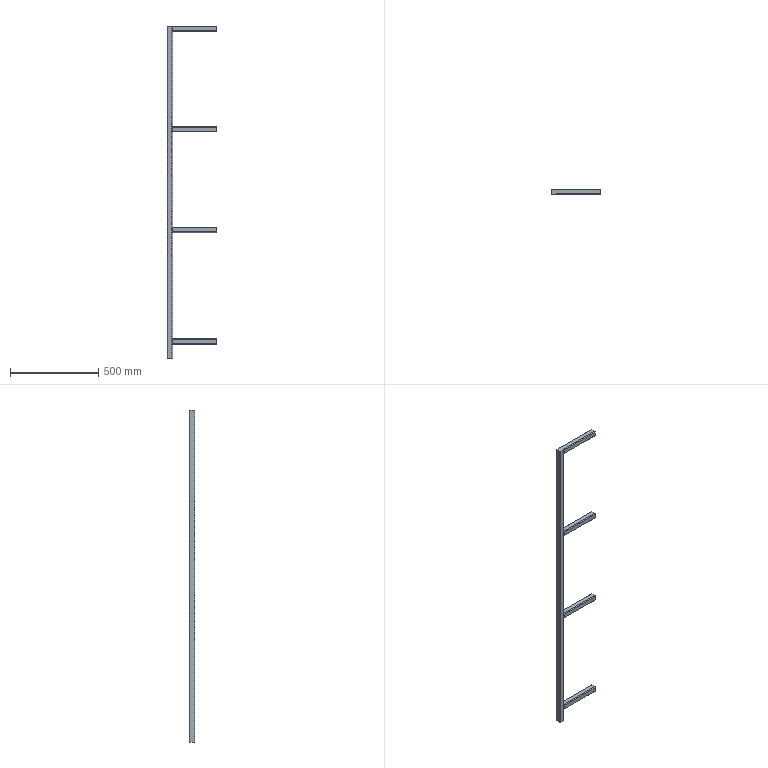Part | SolidWorks | features Extrusion 1, ICE 1 | 1 solid | 56 faces | box 280 x 30 x 1880 mm | volume 2561715 mm3 | plane 36 | cylinder 20 | commonest cylinder face diameters 7 x20
STEP:
#1=CARTESIAN_POINT('',(30.,-26.5,78.062));
#2=VERTEX_POINT('',#1);
#3=CARTESIAN_POINT('',(30.,-3.5,78.062));
#4=VERTEX_POINT('',#3);
#5=CARTESIAN_POINT('',(30.,-3.5,78.062));
#6=DIRECTION('',(0.,1.,0.));
#7=VECTOR('',#6,1000.);
#8=LINE('',#5,#7);
#9=EDGE_CURVE('',#2,#4,#8,.T.);
#10=ORIENTED_EDGE('',*,*,#9,.F.);
#11=CARTESIAN_POINT('',(30.,-26.5,0.));
#12=VERTEX_POINT('',#11);
#13=CARTESIAN_POINT('',(30.,-26.5,1880.));
#14=DIRECTION('',(0.,0.,-1.));
#15=VECTOR('',#14,1000.);
#16=LINE('',#13,#15);
#17=EDGE_CURVE('',#2,#12,#16,.T.);
#18=ORIENTED_EDGE('',*,*,#17,.T.);
#19=CARTESIAN_POINT('',(30.,-3.5,0.));
#20=VERTEX_POINT('',#19);
#21=CARTESIAN_POINT('',(30.,-3.5,0.));
#22=DIRECTION('',(0.,1.,0.));
#23=VECTOR('',#22,1000.);
#24=LINE('',#21,#23);
#25=EDGE_CURVE('',#12,#20,#24,.T.);
#26=ORIENTED_EDGE('',*,*,#25,.T.);
#27=CARTESIAN_POINT('',(30.,-3.5,1880.));
#28=DIRECTION('',(0.,0.,-1.));
#29=VECTOR('',#28,1000.);
#30=LINE('',#27,#29);
#31=EDGE_CURVE('',#4,#20,#30,.T.);
#32=ORIENTED_EDGE('',*,*,#31,.F.);
#33=EDGE_LOOP('',(#10,#18,#26,#32));
#34=FACE_OUTER_BOUND('',#33,.T.);
#35=CARTESIAN_POINT('',(30.,-3.5,1880.));
#36=DIRECTION('',(-1.,0.,0.));
#37=DIRECTION('',(0.,-1.,0.));
#38=AXIS2_PLACEMENT_3D('',#35,#36,#37);
#39=PLANE('',#38);
#40=ADVANCED_FACE('',(#34),#39,.F.);
#41=CARTESIAN_POINT('',(30.,-3.5,108.062));
#42=VERTEX_POINT('',#41);
#43=CARTESIAN_POINT('',(30.,-26.5,108.062));
#44=VERTEX_POINT('',#43);
#45=CARTESIAN_POINT('',(30.,-3.5,108.062));
#46=DIRECTION('',(0.,-1.,0.));
#47=VECTOR('',#46,1000.);
#48=LINE('',#45,#47);
#49=EDGE_CURVE('',#42,#44,#48,.T.);
#50=ORIENTED_EDGE('',*,*,#49,.F.);
#51=CARTESIAN_POINT('',(30.,-3.5,710.369));
#52=VERTEX_POINT('',#51);
#53=CARTESIAN_POINT('',(30.,-3.5,1880.));
#54=DIRECTION('',(0.,0.,-1.));
#55=VECTOR('',#54,1000.);
#56=LINE('',#53,#55);
#57=EDGE_CURVE('',#52,#42,#56,.T.);
#58=ORIENTED_EDGE('',*,*,#57,.F.);
#59=CARTESIAN_POINT('',(30.,-26.5,710.369));
#60=VERTEX_POINT('',#59);
#61=CARTESIAN_POINT('',(30.,-3.5,710.369));
#62=DIRECTION('',(0.,1.,0.));
#63=VECTOR('',#62,1000.);
#64=LINE('',#61,#63);
#65=EDGE_CURVE('',#60,#52,#64,.T.);
#66=ORIENTED_EDGE('',*,*,#65,.F.);
#67=CARTESIAN_POINT('',(30.,-26.5,1880.));
#68=DIRECTION('',(0.,0.,-1.));
#69=VECTOR('',#68,1000.);
#70=LINE('',#67,#69);
#71=EDGE_CURVE('',#60,#44,#70,.T.);
#72=ORIENTED_EDGE('',*,*,#71,.T.);
#73=EDGE_LOOP('',(#50,#58,#66,#72));
#74=FACE_OUTER_BOUND('',#73,.T.);
#75=CARTESIAN_POINT('',(30.,-3.5,1880.));
#76=DIRECTION('',(-1.,0.,0.));
#77=DIRECTION('',(0.,-1.,0.));
#78=AXIS2_PLACEMENT_3D('',#75,#76,#77);
#79=PLANE('',#78);
#80=ADVANCED_FACE('',(#74),#79,.F.);
#81=CARTESIAN_POINT('',(30.,-3.5,740.369));
#82=VERTEX_POINT('',#81);
#83=CARTESIAN_POINT('',(30.,-26.5,740.369));
#84=VERTEX_POINT('',#83);
#85=CARTESIAN_POINT('',(30.,-3.5,740.369));
#86=DIRECTION('',(0.,-1.,0.));
#87=VECTOR('',#86,1000.);
#88=LINE('',#85,#87);
#89=EDGE_CURVE('',#82,#84,#88,.T.);
#90=ORIENTED_EDGE('',*,*,#89,.F.);
#91=CARTESIAN_POINT('',(30.,-3.5,1280.242));
#92=VERTEX_POINT('',#91);
#93=CARTESIAN_POINT('',(30.,-3.5,1880.));
#94=DIRECTION('',(0.,0.,-1.));
#95=VECTOR('',#94,1000.);
#96=LINE('',#93,#95);
#97=EDGE_CURVE('',#92,#82,#96,.T.);
#98=ORIENTED_EDGE('',*,*,#97,.F.);
#99=CARTESIAN_POINT('',(30.,-26.5,1280.242));
#100=VERTEX_POINT('',#99);
#101=CARTESIAN_POINT('',(30.,-3.5,1280.242));
#102=DIRECTION('',(0.,1.,0.));
#103=VECTOR('',#102,1000.);
#104=LINE('',#101,#103);
#105=EDGE_CURVE('',#100,#92,#104,.T.);
#106=ORIENTED_EDGE('',*,*,#105,.F.);
#107=CARTESIAN_POINT('',(30.,-26.5,1880.));
#108=DIRECTION('',(0.,0.,-1.));
#109=VECTOR('',#108,1000.);
#110=LINE('',#107,#109);
#111=EDGE_CURVE('',#100,#84,#110,.T.);
#112=ORIENTED_EDGE('',*,*,#111,.T.);
#113=EDGE_LOOP('',(#90,#98,#106,#112));
#114=FACE_OUTER_BOUND('',#113,.T.);
#115=CARTESIAN_POINT('',(30.,-3.5,1880.));
#116=DIRECTION('',(-1.,0.,0.));
#117=DIRECTION('',(0.,-1.,0.));
#118=AXIS2_PLACEMENT_3D('',#115,#116,#117);
#119=PLANE('',#118);
#120=ADVANCED_FACE('',(#114),#119,.F.);
#121=CARTESIAN_POINT('',(30.,-3.5,1310.242));
#122=VERTEX_POINT('',#121);
#123=CARTESIAN_POINT('',(30.,-26.5,1310.242));
#124=VERTEX_POINT('',#123);
#125=CARTESIAN_POINT('',(30.,-3.5,1310.242));
#126=DIRECTION('',(0.,-1.,0.));
#127=VECTOR('',#126,1000.);
#128=LINE('',#125,#127);
#129=EDGE_CURVE('',#122,#124,#128,.T.);
#130=ORIENTED_EDGE('',*,*,#129,.F.);
#131=CARTESIAN_POINT('',(30.,-3.5,1850.));
#132=VERTEX_POINT('',#131);
#133=CARTESIAN_POINT('',(30.,-3.5,1880.));
#134=DIRECTION('',(0.,0.,-1.));
#135=VECTOR('',#134,1000.);
#136=LINE('',#133,#135);
#137=EDGE_CURVE('',#132,#122,#136,.T.);
#138=ORIENTED_EDGE('',*,*,#137,.F.);
#139=CARTESIAN_POINT('',(30.,-26.5,1850.));
#140=VERTEX_POINT('',#139);
#141=CARTESIAN_POINT('',(30.,-3.5,1850.));
#142=DIRECTION('',(0.,1.,0.));
#143=VECTOR('',#142,1000.);
#144=LINE('',#141,#143);
#145=EDGE_CURVE('',#140,#132,#144,.T.);
#146=ORIENTED_EDGE('',*,*,#145,.F.);
#147=CARTESIAN_POINT('',(30.,-26.5,1880.));
#148=DIRECTION('',(0.,0.,-1.));
#149=VECTOR('',#148,1000.);
#150=LINE('',#147,#149);
#151=EDGE_CURVE('',#140,#124,#150,.T.);
#152=ORIENTED_EDGE('',*,*,#151,.T.);
#153=EDGE_LOOP('',(#130,#138,#146,#152));
#154=FACE_OUTER_BOUND('',#153,.T.);
#155=CARTESIAN_POINT('',(30.,-3.5,1880.));
#156=DIRECTION('',(-1.,0.,0.));
#157=DIRECTION('',(0.,-1.,0.));
#158=AXIS2_PLACEMENT_3D('',#155,#156,#157);
#159=PLANE('',#158);
#160=ADVANCED_FACE('',(#154),#159,.F.);
#161=CARTESIAN_POINT('',(26.5,-30.,0.));
#162=VERTEX_POINT('',#161);
#163=CARTESIAN_POINT('',(26.5,-26.5,0.));
#164=DIRECTION('',(0.,0.,1.));
#165=DIRECTION('',(1.,0.,0.));
#166=AXIS2_PLACEMENT_3D('',#163,#164,#165);
#167=CIRCLE('',#166,3.5);
#168=EDGE_CURVE('',#162,#12,#167,.T.);
#169=ORIENTED_EDGE('',*,*,#168,.T.);
#170=ORIENTED_EDGE('',*,*,#17,.F.);
#171=CARTESIAN_POINT('',(30.,-26.5,1880.));
#172=DIRECTION('',(0.,0.,-1.));
#173=VECTOR('',#172,1000.);
#174=LINE('',#171,#173);
#175=EDGE_CURVE('',#44,#2,#174,.T.);
#176=ORIENTED_EDGE('',*,*,#175,.F.);
#177=ORIENTED_EDGE('',*,*,#71,.F.);
#178=CARTESIAN_POINT('',(30.,-26.5,1880.));
#179=DIRECTION('',(0.,0.,-1.));
#180=VECTOR('',#179,1000.);
#181=LINE('',#178,#180);
#182=EDGE_CURVE('',#84,#60,#181,.T.);
#183=ORIENTED_EDGE('',*,*,#182,.F.);
#184=ORIENTED_EDGE('',*,*,#111,.F.);
#185=CARTESIAN_POINT('',(30.,-26.5,1880.));
#186=DIRECTION('',(0.,0.,-1.));
#187=VECTOR('',#186,1000.);
#188=LINE('',#185,#187);
#189=EDGE_CURVE('',#124,#100,#188,.T.);
#190=ORIENTED_EDGE('',*,*,#189,.F.);
#191=ORIENTED_EDGE('',*,*,#151,.F.);
#192=CARTESIAN_POINT('',(30.,-26.5,1880.));
#193=VERTEX_POINT('',#192);
#194=CARTESIAN_POINT('',(30.,-26.5,1880.));
#195=DIRECTION('',(0.,0.,-1.));
#196=VECTOR('',#195,1000.);
#197=LINE('',#194,#196);
#198=EDGE_CURVE('',#193,#140,#197,.T.);
#199=ORIENTED_EDGE('',*,*,#198,.F.);
#200=CARTESIAN_POINT('',(26.5,-30.,1880.));
#201=VERTEX_POINT('',#200);
#202=CARTESIAN_POINT('',(26.5,-26.5,1880.));
#203=DIRECTION('',(0.,0.,1.));
#204=DIRECTION('',(1.,0.,0.));
#205=AXIS2_PLACEMENT_3D('',#202,#203,#204);
#206=CIRCLE('',#205,3.5);
#207=EDGE_CURVE('',#201,#193,#206,.T.);
#208=ORIENTED_EDGE('',*,*,#207,.F.);
#209=CARTESIAN_POINT('',(26.5,-30.,1880.));
#210=DIRECTION('',(0.,0.,-1.));
#211=VECTOR('',#210,1000.);
#212=LINE('',#209,#211);
#213=EDGE_CURVE('',#201,#162,#212,.T.);
#214=ORIENTED_EDGE('',*,*,#213,.T.);
#215=EDGE_LOOP('',(#169,#170,#176,#177,#183,#184,#190,#191,#199,#208,#214));
#216=FACE_OUTER_BOUND('',#215,.T.);
#217=CARTESIAN_POINT('',(26.5,-26.5,1880.));
#218=DIRECTION('',(0.,0.,-1.));
#219=DIRECTION('',(-1.,0.,0.));
#220=AXIS2_PLACEMENT_3D('',#217,#218,#219);
#221=CYLINDRICAL_SURFACE('',#220,3.5);
#222=ADVANCED_FACE('',(#216),#221,.T.);
#223=CARTESIAN_POINT('',(26.5,0.,0.));
#224=VERTEX_POINT('',#223);
#225=CARTESIAN_POINT('',(26.5,-3.5,0.));
#226=DIRECTION('',(0.,0.,1.));
#227=DIRECTION('',(-1.,0.,0.));
#228=AXIS2_PLACEMENT_3D('',#225,#226,#227);
#229=CIRCLE('',#228,3.5);
#230=EDGE_CURVE('',#20,#224,#229,.T.);
#231=ORIENTED_EDGE('',*,*,#230,.T.);
#232=CARTESIAN_POINT('',(26.5,0.,1880.));
#233=VERTEX_POINT('',#232);
#234=CARTESIAN_POINT('',(26.5,0.,1880.));
#235=DIRECTION('',(0.,0.,-1.));
#236=VECTOR('',#235,1000.);
#237=LINE('',#234,#236);
#238=EDGE_CURVE('',#233,#224,#237,.T.);
#239=ORIENTED_EDGE('',*,*,#238,.F.);
#240=CARTESIAN_POINT('',(30.,-3.5,1880.));
#241=VERTEX_POINT('',#240);
#242=CARTESIAN_POINT('',(26.5,-3.5,1880.));
#243=DIRECTION('',(0.,0.,1.));
#244=DIRECTION('',(-1.,0.,0.));
#245=AXIS2_PLACEMENT_3D('',#242,#243,#244);
#246=CIRCLE('',#245,3.5);
#247=EDGE_CURVE('',#241,#233,#246,.T.);
#248=ORIENTED_EDGE('',*,*,#247,.F.);
#249=CARTESIAN_POINT('',(30.,-3.5,1880.));
#250=DIRECTION('',(0.,0.,-1.));
#251=VECTOR('',#250,1000.);
#252=LINE('',#249,#251);
#253=EDGE_CURVE('',#241,#132,#252,.T.);
#254=ORIENTED_EDGE('',*,*,#253,.T.);
#255=ORIENTED_EDGE('',*,*,#137,.T.);
#256=CARTESIAN_POINT('',(30.,-3.5,1880.));
#257=DIRECTION('',(0.,0.,-1.));
#258=VECTOR('',#257,1000.);
#259=LINE('',#256,#258);
#260=EDGE_CURVE('',#122,#92,#259,.T.);
#261=ORIENTED_EDGE('',*,*,#260,.T.);
#262=ORIENTED_EDGE('',*,*,#97,.T.);
#263=CARTESIAN_POINT('',(30.,-3.5,1880.));
#264=DIRECTION('',(0.,0.,-1.));
#265=VECTOR('',#264,1000.);
#266=LINE('',#263,#265);
#267=EDGE_CURVE('',#82,#52,#266,.T.);
#268=ORIENTED_EDGE('',*,*,#267,.T.);
#269=ORIENTED_EDGE('',*,*,#57,.T.);
#270=CARTESIAN_POINT('',(30.,-3.5,1880.));
#271=DIRECTION('',(0.,0.,-1.));
#272=VECTOR('',#271,1000.);
#273=LINE('',#270,#272);
#274=EDGE_CURVE('',#42,#4,#273,.T.);
#275=ORIENTED_EDGE('',*,*,#274,.T.);
#276=ORIENTED_EDGE('',*,*,#31,.T.);
#277=EDGE_LOOP('',(#231,#239,#248,#254,#255,#261,#262,#268,#269,#275,#276));
#278=FACE_OUTER_BOUND('',#277,.T.);
#279=CARTESIAN_POINT('',(26.5,-3.5,1880.));
#280=DIRECTION('',(0.,0.,-1.));
#281=DIRECTION('',(-1.,0.,0.));
#282=AXIS2_PLACEMENT_3D('',#279,#280,#281);
#283=CYLINDRICAL_SURFACE('',#282,3.5);
#284=ADVANCED_FACE('',(#278),#283,.T.);
#285=CARTESIAN_POINT('',(3.5,0.,0.));
#286=VERTEX_POINT('',#285);
#287=CARTESIAN_POINT('',(3.5,0.,0.));
#288=DIRECTION('',(-1.,0.,0.));
#289=VECTOR('',#288,1000.);
#290=LINE('',#287,#289);
#291=EDGE_CURVE('',#224,#286,#290,.T.);
#292=ORIENTED_EDGE('',*,*,#291,.T.);
#293=CARTESIAN_POINT('',(3.5,0.,1880.));
#294=VERTEX_POINT('',#293);
#295=CARTESIAN_POINT('',(3.5,0.,1880.));
#296=DIRECTION('',(0.,0.,-1.));
#297=VECTOR('',#296,1000.);
#298=LINE('',#295,#297);
#299=EDGE_CURVE('',#294,#286,#298,.T.);
#300=ORIENTED_EDGE('',*,*,#299,.F.);
#301=CARTESIAN_POINT('',(3.5,0.,1880.));
#302=DIRECTION('',(-1.,0.,0.));
#303=VECTOR('',#302,1000.);
#304=LINE('',#301,#303);
#305=EDGE_CURVE('',#233,#294,#304,.T.);
#306=ORIENTED_EDGE('',*,*,#305,.F.);
#307=ORIENTED_EDGE('',*,*,#238,.T.);
#308=EDGE_LOOP('',(#292,#300,#306,#307));
#309=FACE_OUTER_BOUND('',#308,.T.);
#310=CARTESIAN_POINT('',(3.5,0.,1880.));
#311=DIRECTION('',(0.,-1.,0.));
#312=DIRECTION('',(0.,0.,-1.));
#313=AXIS2_PLACEMENT_3D('',#310,#311,#312);
#314=PLANE('',#313);
#315=ADVANCED_FACE('',(#309),#314,.F.);
#316=CARTESIAN_POINT('',(0.,-3.5,0.));
#317=VERTEX_POINT('',#316);
#318=CARTESIAN_POINT('',(3.5,-3.5,0.));
#319=DIRECTION('',(0.,0.,1.));
#320=DIRECTION('',(1.,0.,0.));
#321=AXIS2_PLACEMENT_3D('',#318,#319,#320);
#322=CIRCLE('',#321,3.5);
#323=EDGE_CURVE('',#286,#317,#322,.T.);
#324=ORIENTED_EDGE('',*,*,#323,.T.);
#325=CARTESIAN_POINT('',(0.,-3.5,1880.));
#326=VERTEX_POINT('',#325);
#327=CARTESIAN_POINT('',(0.,-3.5,1880.));
#328=DIRECTION('',(0.,0.,-1.));
#329=VECTOR('',#328,1000.);
#330=LINE('',#327,#329);
#331=EDGE_CURVE('',#326,#317,#330,.T.);
#332=ORIENTED_EDGE('',*,*,#331,.F.);
#333=CARTESIAN_POINT('',(3.5,-3.5,1880.));
#334=DIRECTION('',(0.,0.,1.));
#335=DIRECTION('',(1.,0.,0.));
#336=AXIS2_PLACEMENT_3D('',#333,#334,#335);
#337=CIRCLE('',#336,3.5);
#338=EDGE_CURVE('',#294,#326,#337,.T.);
#339=ORIENTED_EDGE('',*,*,#338,.F.);
#340=ORIENTED_EDGE('',*,*,#299,.T.);
#341=EDGE_LOOP('',(#324,#332,#339,#340));
#342=FACE_OUTER_BOUND('',#341,.T.);
#343=CARTESIAN_POINT('',(3.5,-3.5,1880.));
#344=DIRECTION('',(0.,0.,-1.));
#345=DIRECTION('',(-1.,0.,0.));
#346=AXIS2_PLACEMENT_3D('',#343,#344,#345);
#347=CYLINDRICAL_SURFACE('',#346,3.5);
#348=ADVANCED_FACE('',(#342),#347,.T.);
#349=CARTESIAN_POINT('',(0.,-26.5,0.));
#350=VERTEX_POINT('',#349);
#351=CARTESIAN_POINT('',(0.,-3.5,0.));
#352=DIRECTION('',(0.,-1.,0.));
#353=VECTOR('',#352,1000.);
#354=LINE('',#351,#353);
#355=EDGE_CURVE('',#317,#350,#354,.T.);
#356=ORIENTED_EDGE('',*,*,#355,.T.);
#357=CARTESIAN_POINT('',(0.,-26.5,1880.));
#358=VERTEX_POINT('',#357);
#359=CARTESIAN_POINT('',(0.,-26.5,1880.));
#360=DIRECTION('',(0.,0.,-1.));
#361=VECTOR('',#360,1000.);
#362=LINE('',#359,#361);
#363=EDGE_CURVE('',#358,#350,#362,.T.);
#364=ORIENTED_EDGE('',*,*,#363,.F.);
#365=CARTESIAN_POINT('',(0.,-3.5,1880.));
#366=DIRECTION('',(0.,-1.,0.));
#367=VECTOR('',#366,1000.);
#368=LINE('',#365,#367);
#369=EDGE_CURVE('',#326,#358,#368,.T.);
#370=ORIENTED_EDGE('',*,*,#369,.F.);
#371=ORIENTED_EDGE('',*,*,#331,.T.);
#372=EDGE_LOOP('',(#356,#364,#370,#371));
#373=FACE_OUTER_BOUND('',#372,.T.);
#374=CARTESIAN_POINT('',(0.,-3.5,1880.));
#375=DIRECTION('',(1.,0.,0.));
#376=DIRECTION('',(0.,0.,-1.));
#377=AXIS2_PLACEMENT_3D('',#374,#375,#376);
#378=PLANE('',#377);
#379=ADVANCED_FACE('',(#373),#378,.F.);
#380=CARTESIAN_POINT('',(3.5,-30.,0.));
#381=VERTEX_POINT('',#380);
#382=CARTESIAN_POINT('',(3.5,-26.5,0.));
#383=DIRECTION('',(0.,0.,1.));
#384=DIRECTION('',(1.,0.,0.));
#385=AXIS2_PLACEMENT_3D('',#382,#383,#384);
#386=CIRCLE('',#385,3.5);
#387=EDGE_CURVE('',#350,#381,#386,.T.);
#388=ORIENTED_EDGE('',*,*,#387,.T.);
#389=CARTESIAN_POINT('',(3.5,-30.,1880.));
#390=VERTEX_POINT('',#389);
#391=CARTESIAN_POINT('',(3.5,-30.,1880.));
#392=DIRECTION('',(0.,0.,-1.));
#393=VECTOR('',#392,1000.);
#394=LINE('',#391,#393);
#395=EDGE_CURVE('',#390,#381,#394,.T.);
#396=ORIENTED_EDGE('',*,*,#395,.F.);
#397=CARTESIAN_POINT('',(3.5,-26.5,1880.));
#398=DIRECTION('',(0.,0.,1.));
#399=DIRECTION('',(1.,0.,0.));
#400=AXIS2_PLACEMENT_3D('',#397,#398,#399);
#401=CIRCLE('',#400,3.5);
#402=EDGE_CURVE('',#358,#390,#401,.T.);
#403=ORIENTED_EDGE('',*,*,#402,.F.);
#404=ORIENTED_EDGE('',*,*,#363,.T.);
#405=EDGE_LOOP('',(#388,#396,#403,#404));
#406=FACE_OUTER_BOUND('',#405,.T.);
#407=CARTESIAN_POINT('',(3.5,-26.5,1880.));
#408=DIRECTION('',(0.,0.,-1.));
#409=DIRECTION('',(-1.,0.,0.));
#410=AXIS2_PLACEMENT_3D('',#407,#408,#409);
#411=CYLINDRICAL_SURFACE('',#410,3.5);
#412=ADVANCED_FACE('',(#406),#411,.T.);
#413=CARTESIAN_POINT('',(3.5,-30.,0.));
#414=DIRECTION('',(1.,0.,0.));
#415=VECTOR('',#414,1000.);
#416=LINE('',#413,#415);
#417=EDGE_CURVE('',#381,#162,#416,.T.);
#418=ORIENTED_EDGE('',*,*,#417,.T.);
#419=ORIENTED_EDGE('',*,*,#213,.F.);
#420=CARTESIAN_POINT('',(3.5,-30.,1880.));
#421=DIRECTION('',(1.,0.,0.));
#422=VECTOR('',#421,1000.);
#423=LINE('',#420,#422);
#424=EDGE_CURVE('',#390,#201,#423,.T.);
#425=ORIENTED_EDGE('',*,*,#424,.F.);
#426=ORIENTED_EDGE('',*,*,#395,.T.);
#427=EDGE_LOOP('',(#418,#419,#425,#426));
#428=FACE_OUTER_BOUND('',#427,.T.);
#429=CARTESIAN_POINT('',(3.5,-30.,1880.));
#430=DIRECTION('',(0.,1.,0.));
#431=DIRECTION('',(0.,0.,1.));
#432=AXIS2_PLACEMENT_3D('',#429,#430,#431);
#433=PLANE('',#432);
#434=ADVANCED_FACE('',(#428),#433,.F.);
#435=ORIENTED_EDGE('',*,*,#207,.T.);
#436=CARTESIAN_POINT('',(280.,-26.5,1880.));
#437=VERTEX_POINT('',#436);
#438=CARTESIAN_POINT('',(280.,-26.5,1880.));
#439=DIRECTION('',(-1.,0.,0.));
#440=VECTOR('',#439,1000.);
#441=LINE('',#438,#440);
#442=EDGE_CURVE('',#437,#193,#441,.T.);
#443=ORIENTED_EDGE('',*,*,#442,.F.);
#444=CARTESIAN_POINT('',(280.,-3.5,1880.));
#445=VERTEX_POINT('',#444);
#446=CARTESIAN_POINT('',(280.,-3.5,1880.));
#447=DIRECTION('',(0.,-1.,0.));
#448=VECTOR('',#447,1000.);
#449=LINE('',#446,#448);
#450=EDGE_CURVE('',#445,#437,#449,.T.);
#451=ORIENTED_EDGE('',*,*,#450,.F.);
#452=CARTESIAN_POINT('',(280.,-3.5,1880.));
#453=DIRECTION('',(-1.,0.,0.));
#454=VECTOR('',#453,1000.);
#455=LINE('',#452,#454);
#456=EDGE_CURVE('',#445,#241,#455,.T.);
#457=ORIENTED_EDGE('',*,*,#456,.T.);
#458=ORIENTED_EDGE('',*,*,#247,.T.);
#459=ORIENTED_EDGE('',*,*,#305,.T.);
#460=ORIENTED_EDGE('',*,*,#338,.T.);
#461=ORIENTED_EDGE('',*,*,#369,.T.);
#462=ORIENTED_EDGE('',*,*,#402,.T.);
#463=ORIENTED_EDGE('',*,*,#424,.T.);
#464=EDGE_LOOP('',(#435,#443,#451,#457,#458,#459,#460,#461,#462,#463));
#465=FACE_OUTER_BOUND('',#464,.T.);
#466=CARTESIAN_POINT('',(26.5,-26.5,1880.));
#467=DIRECTION('',(0.,0.,1.));
#468=DIRECTION('',(1.,0.,0.));
#469=AXIS2_PLACEMENT_3D('',#466,#467,#468);
#470=PLANE('',#469);
#471=ADVANCED_FACE('',(#465),#470,.T.);
#472=ORIENTED_EDGE('',*,*,#168,.F.);
#473=ORIENTED_EDGE('',*,*,#417,.F.);
#474=ORIENTED_EDGE('',*,*,#387,.F.);
#475=ORIENTED_EDGE('',*,*,#355,.F.);
#476=ORIENTED_EDGE('',*,*,#323,.F.);
#477=ORIENTED_EDGE('',*,*,#291,.F.);
#478=ORIENTED_EDGE('',*,*,#230,.F.);
#479=ORIENTED_EDGE('',*,*,#25,.F.);
#480=EDGE_LOOP('',(#472,#473,#474,#475,#476,#477,#478,#479));
#481=FACE_OUTER_BOUND('',#480,.T.);
#482=CARTESIAN_POINT('',(26.5,-26.5,0.));
#483=DIRECTION('',(0.,0.,1.));
#484=DIRECTION('',(1.,0.,0.));
#485=AXIS2_PLACEMENT_3D('',#482,#483,#484);
#486=PLANE('',#485);
#487=ADVANCED_FACE('',(#481),#486,.F.);
#488=CARTESIAN_POINT('',(30.,-30.,1876.5));
#489=VERTEX_POINT('',#488);
#490=CARTESIAN_POINT('',(30.,-26.5,1876.5));
#491=DIRECTION('',(1.,0.,0.));
#492=DIRECTION('',(0.,1.,0.));
#493=AXIS2_PLACEMENT_3D('',#490,#491,#492);
#494=CIRCLE('',#493,3.5);
#495=EDGE_CURVE('',#193,#489,#494,.T.);
#496=ORIENTED_EDGE('',*,*,#495,.F.);
#497=ORIENTED_EDGE('',*,*,#198,.T.);
#498=CARTESIAN_POINT('',(30.,-30.,1853.5));
#499=VERTEX_POINT('',#498);
#500=CARTESIAN_POINT('',(30.,-26.5,1853.5));
#501=DIRECTION('',(1.,0.,0.));
#502=DIRECTION('',(0.,1.,0.));
#503=AXIS2_PLACEMENT_3D('',#500,#501,#502);
#504=CIRCLE('',#503,3.5);
#505=EDGE_CURVE('',#499,#140,#504,.T.);
#506=ORIENTED_EDGE('',*,*,#505,.F.);
#507=CARTESIAN_POINT('',(30.,-30.,1876.5));
#508=DIRECTION('',(0.,0.,-1.));
#509=VECTOR('',#508,1000.);
#510=LINE('',#507,#509);
#511=EDGE_CURVE('',#489,#499,#510,.T.);
#512=ORIENTED_EDGE('',*,*,#511,.F.);
#513=EDGE_LOOP('',(#496,#497,#506,#512));
#514=FACE_OUTER_BOUND('',#513,.T.);
#515=CARTESIAN_POINT('',(30.,-26.5,1876.5));
#516=DIRECTION('',(1.,0.,0.));
#517=DIRECTION('',(0.,1.,0.));
#518=AXIS2_PLACEMENT_3D('',#515,#516,#517);
#519=PLANE('',#518);
#520=ADVANCED_FACE('',(#514),#519,.F.);
#521=ORIENTED_EDGE('',*,*,#495,.T.);
#522=CARTESIAN_POINT('',(280.,-30.,1876.5));
#523=VERTEX_POINT('',#522);
#524=CARTESIAN_POINT('',(280.,-30.,1876.5));
#525=DIRECTION('',(-1.,0.,0.));
#526=VECTOR('',#525,1000.);
#527=LINE('',#524,#526);
#528=EDGE_CURVE('',#523,#489,#527,.T.);
#529=ORIENTED_EDGE('',*,*,#528,.F.);
#530=CARTESIAN_POINT('',(280.,-26.5,1876.5));
#531=DIRECTION('',(1.,0.,0.));
#532=DIRECTION('',(0.,1.,0.));
#533=AXIS2_PLACEMENT_3D('',#530,#531,#532);
#534=CIRCLE('',#533,3.5);
#535=EDGE_CURVE('',#437,#523,#534,.T.);
#536=ORIENTED_EDGE('',*,*,#535,.F.);
#537=ORIENTED_EDGE('',*,*,#442,.T.);
#538=EDGE_LOOP('',(#521,#529,#536,#537));
#539=FACE_OUTER_BOUND('',#538,.T.);
#540=CARTESIAN_POINT('',(280.,-26.5,1876.5));
#541=DIRECTION('',(-1.,0.,0.));
#542=DIRECTION('',(0.,-1.,0.));
#543=AXIS2_PLACEMENT_3D('',#540,#541,#542);
#544=CYLINDRICAL_SURFACE('',#543,3.5);
#545=ADVANCED_FACE('',(#539),#544,.T.);
#546=ORIENTED_EDGE('',*,*,#511,.T.);
#547=CARTESIAN_POINT('',(280.,-30.,1853.5));
#548=VERTEX_POINT('',#547);
#549=CARTESIAN_POINT('',(280.,-30.,1853.5));
#550=DIRECTION('',(-1.,0.,0.));
#551=VECTOR('',#550,1000.);
#552=LINE('',#549,#551);
#553=EDGE_CURVE('',#548,#499,#552,.T.);
#554=ORIENTED_EDGE('',*,*,#553,.F.);
#555=CARTESIAN_POINT('',(280.,-30.,1876.5));
#556=DIRECTION('',(0.,0.,-1.));
#557=VECTOR('',#556,1000.);
#558=LINE('',#555,#557);
#559=EDGE_CURVE('',#523,#548,#558,.T.);
#560=ORIENTED_EDGE('',*,*,#559,.F.);
#561=ORIENTED_EDGE('',*,*,#528,.T.);
#562=EDGE_LOOP('',(#546,#554,#560,#561));
#563=FACE_OUTER_BOUND('',#562,.T.);
#564=CARTESIAN_POINT('',(280.,-30.,1876.5));
#565=DIRECTION('',(0.,1.,0.));
#566=DIRECTION('',(-1.,0.,0.));
#567=AXIS2_PLACEMENT_3D('',#564,#565,#566);
#568=PLANE('',#567);
#569=ADVANCED_FACE('',(#563),#568,.F.);
#570=ORIENTED_EDGE('',*,*,#505,.T.);
#571=CARTESIAN_POINT('',(280.,-26.5,1850.));
#572=VERTEX_POINT('',#571);
#573=CARTESIAN_POINT('',(280.,-26.5,1850.));
#574=DIRECTION('',(-1.,0.,0.));
#575=VECTOR('',#574,1000.);
#576=LINE('',#573,#575);
#577=EDGE_CURVE('',#572,#140,#576,.T.);
#578=ORIENTED_EDGE('',*,*,#577,.F.);
#579=CARTESIAN_POINT('',(280.,-26.5,1853.5));
#580=DIRECTION('',(1.,0.,0.));
#581=DIRECTION('',(0.,1.,0.));
#582=AXIS2_PLACEMENT_3D('',#579,#580,#581);
#583=CIRCLE('',#582,3.5);
#584=EDGE_CURVE('',#548,#572,#583,.T.);
#585=ORIENTED_EDGE('',*,*,#584,.F.);
#586=ORIENTED_EDGE('',*,*,#553,.T.);
#587=EDGE_LOOP('',(#570,#578,#585,#586));
#588=FACE_OUTER_BOUND('',#587,.T.);
#589=CARTESIAN_POINT('',(280.,-26.5,1853.5));
#590=DIRECTION('',(-1.,0.,0.));
#591=DIRECTION('',(0.,-1.,0.));
#592=AXIS2_PLACEMENT_3D('',#589,#590,#591);
#593=CYLINDRICAL_SURFACE('',#592,3.5);
#594=ADVANCED_FACE('',(#588),#593,.T.);
#595=ORIENTED_EDGE('',*,*,#145,.T.);
#596=CARTESIAN_POINT('',(280.,-3.5,1850.));
#597=VERTEX_POINT('',#596);
#598=CARTESIAN_POINT('',(280.,-3.5,1850.));
#599=DIRECTION('',(-1.,0.,0.));
#600=VECTOR('',#599,1000.);
#601=LINE('',#598,#600);
#602=EDGE_CURVE('',#597,#132,#601,.T.);
#603=ORIENTED_EDGE('',*,*,#602,.F.);
#604=CARTESIAN_POINT('',(280.,-3.5,1850.));
#605=DIRECTION('',(0.,1.,0.));
#606=VECTOR('',#605,1000.);
#607=LINE('',#604,#606);
#608=EDGE_CURVE('',#572,#597,#607,.T.);
#609=ORIENTED_EDGE('',*,*,#608,.F.);
#610=ORIENTED_EDGE('',*,*,#577,.T.);
#611=EDGE_LOOP('',(#595,#603,#609,#610));
#612=FACE_OUTER_BOUND('',#611,.T.);
#613=CARTESIAN_POINT('',(280.,-3.5,1850.));
#614=DIRECTION('',(0.,0.,1.));
#615=DIRECTION('',(1.,0.,0.));
#616=AXIS2_PLACEMENT_3D('',#613,#614,#615);
#617=PLANE('',#616);
#618=ADVANCED_FACE('',(#612),#617,.F.);
#619=CARTESIAN_POINT('',(30.,0.,1853.5));
#620=VERTEX_POINT('',#619);
#621=CARTESIAN_POINT('',(30.,-3.5,1853.5));
#622=DIRECTION('',(1.,0.,0.));
#623=DIRECTION('',(0.,-1.,0.));
#624=AXIS2_PLACEMENT_3D('',#621,#622,#623);
#625=CIRCLE('',#624,3.5);
#626=EDGE_CURVE('',#132,#620,#625,.T.);
#627=ORIENTED_EDGE('',*,*,#626,.T.);
#628=CARTESIAN_POINT('',(280.,0.,1853.5));
#629=VERTEX_POINT('',#628);
#630=CARTESIAN_POINT('',(280.,0.,1853.5));
#631=DIRECTION('',(-1.,0.,0.));
#632=VECTOR('',#631,1000.);
#633=LINE('',#630,#632);
#634=EDGE_CURVE('',#629,#620,#633,.T.);
#635=ORIENTED_EDGE('',*,*,#634,.F.);
#636=CARTESIAN_POINT('',(280.,-3.5,1853.5));
#637=DIRECTION('',(1.,0.,0.));
#638=DIRECTION('',(0.,-1.,0.));
#639=AXIS2_PLACEMENT_3D('',#636,#637,#638);
#640=CIRCLE('',#639,3.5);
#641=EDGE_CURVE('',#597,#629,#640,.T.);
#642=ORIENTED_EDGE('',*,*,#641,.F.);
#643=ORIENTED_EDGE('',*,*,#602,.T.);
#644=EDGE_LOOP('',(#627,#635,#642,#643));
#645=FACE_OUTER_BOUND('',#644,.T.);
#646=CARTESIAN_POINT('',(280.,-3.5,1853.5));
#647=DIRECTION('',(-1.,0.,0.));
#648=DIRECTION('',(0.,-1.,0.));
#649=AXIS2_PLACEMENT_3D('',#646,#647,#648);
#650=CYLINDRICAL_SURFACE('',#649,3.5);
#651=ADVANCED_FACE('',(#645),#650,.T.);
#652=CARTESIAN_POINT('',(30.,0.,1876.5));
#653=VERTEX_POINT('',#652);
#654=CARTESIAN_POINT('',(30.,0.,1876.5));
#655=DIRECTION('',(0.,0.,1.));
#656=VECTOR('',#655,1000.);
#657=LINE('',#654,#656);
#658=EDGE_CURVE('',#620,#653,#657,.T.);
#659=ORIENTED_EDGE('',*,*,#658,.T.);
#660=CARTESIAN_POINT('',(280.,0.,1876.5));
#661=VERTEX_POINT('',#660);
#662=CARTESIAN_POINT('',(280.,0.,1876.5));
#663=DIRECTION('',(-1.,0.,0.));
#664=VECTOR('',#663,1000.);
#665=LINE('',#662,#664);
#666=EDGE_CURVE('',#661,#653,#665,.T.);
#667=ORIENTED_EDGE('',*,*,#666,.F.);
#668=CARTESIAN_POINT('',(280.,0.,1876.5));
#669=DIRECTION('',(0.,0.,1.));
#670=VECTOR('',#669,1000.);
#671=LINE('',#668,#670);
#672=EDGE_CURVE('',#629,#661,#671,.T.);
#673=ORIENTED_EDGE('',*,*,#672,.F.);
#674=ORIENTED_EDGE('',*,*,#634,.T.);
#675=EDGE_LOOP('',(#659,#667,#673,#674));
#676=FACE_OUTER_BOUND('',#675,.T.);
#677=CARTESIAN_POINT('',(280.,0.,1876.5));
#678=DIRECTION('',(0.,-1.,0.));
#679=DIRECTION('',(1.,0.,0.));
#680=AXIS2_PLACEMENT_3D('',#677,#678,#679);
#681=PLANE('',#680);
#682=ADVANCED_FACE('',(#676),#681,.F.);
#683=CARTESIAN_POINT('',(30.,-3.5,1876.5));
#684=DIRECTION('',(1.,0.,0.));
#685=DIRECTION('',(0.,1.,0.));
#686=AXIS2_PLACEMENT_3D('',#683,#684,#685);
#687=CIRCLE('',#686,3.5);
#688=EDGE_CURVE('',#653,#241,#687,.T.);
#689=ORIENTED_EDGE('',*,*,#688,.T.);
#690=ORIENTED_EDGE('',*,*,#456,.F.);
#691=CARTESIAN_POINT('',(280.,-3.5,1876.5));
#692=DIRECTION('',(1.,0.,0.));
#693=DIRECTION('',(0.,1.,0.));
#694=AXIS2_PLACEMENT_3D('',#691,#692,#693);
#695=CIRCLE('',#694,3.5);
#696=EDGE_CURVE('',#661,#445,#695,.T.);
#697=ORIENTED_EDGE('',*,*,#696,.F.);
#698=ORIENTED_EDGE('',*,*,#666,.T.);
#699=EDGE_LOOP('',(#689,#690,#697,#698));
#700=FACE_OUTER_BOUND('',#699,.T.);
#701=CARTESIAN_POINT('',(280.,-3.5,1876.5));
#702=DIRECTION('',(-1.,0.,0.));
#703=DIRECTION('',(0.,-1.,0.));
#704=AXIS2_PLACEMENT_3D('',#701,#702,#703);
#705=CYLINDRICAL_SURFACE('',#704,3.5);
#706=ADVANCED_FACE('',(#700),#705,.T.);
#707=ORIENTED_EDGE('',*,*,#535,.T.);
#708=ORIENTED_EDGE('',*,*,#559,.T.);
#709=ORIENTED_EDGE('',*,*,#584,.T.);
#710=ORIENTED_EDGE('',*,*,#608,.T.);
#711=ORIENTED_EDGE('',*,*,#641,.T.);
#712=ORIENTED_EDGE('',*,*,#672,.T.);
#713=ORIENTED_EDGE('',*,*,#696,.T.);
#714=ORIENTED_EDGE('',*,*,#450,.T.);
#715=EDGE_LOOP('',(#707,#708,#709,#710,#711,#712,#713,#714));
#716=FACE_OUTER_BOUND('',#715,.T.);
#717=CARTESIAN_POINT('',(280.,-26.5,1876.5));
#718=DIRECTION('',(1.,0.,0.));
#719=DIRECTION('',(0.,1.,0.));
#720=AXIS2_PLACEMENT_3D('',#717,#718,#719);
#721=PLANE('',#720);
#722=ADVANCED_FACE('',(#716),#721,.T.);
#723=ORIENTED_EDGE('',*,*,#253,.F.);
#724=ORIENTED_EDGE('',*,*,#688,.F.);
#725=ORIENTED_EDGE('',*,*,#658,.F.);
#726=ORIENTED_EDGE('',*,*,#626,.F.);
#727=EDGE_LOOP('',(#723,#724,#725,#726));
#728=FACE_OUTER_BOUND('',#727,.T.);
#729=CARTESIAN_POINT('',(30.,-26.5,1876.5));
#730=DIRECTION('',(1.,0.,0.));
#731=DIRECTION('',(0.,1.,0.));
#732=AXIS2_PLACEMENT_3D('',#729,#730,#731);
#733=PLANE('',#732);
#734=ADVANCED_FACE('',(#728),#733,.F.);
#735=CARTESIAN_POINT('',(30.,-30.,1306.742));
#736=VERTEX_POINT('',#735);
#737=CARTESIAN_POINT('',(30.,-26.5,1306.742));
#738=DIRECTION('',(1.,0.,0.));
#739=DIRECTION('',(0.,1.,0.));
#740=AXIS2_PLACEMENT_3D('',#737,#738,#739);
#741=CIRCLE('',#740,3.5);
#742=EDGE_CURVE('',#124,#736,#741,.T.);
#743=ORIENTED_EDGE('',*,*,#742,.F.);
#744=ORIENTED_EDGE('',*,*,#189,.T.);
#745=CARTESIAN_POINT('',(30.,-30.,1283.742));
#746=VERTEX_POINT('',#745);
#747=CARTESIAN_POINT('',(30.,-26.5,1283.742));
#748=DIRECTION('',(1.,0.,0.));
#749=DIRECTION('',(0.,1.,0.));
#750=AXIS2_PLACEMENT_3D('',#747,#748,#749);
#751=CIRCLE('',#750,3.5);
#752=EDGE_CURVE('',#746,#100,#751,.T.);
#753=ORIENTED_EDGE('',*,*,#752,.F.);
#754=CARTESIAN_POINT('',(30.,-30.,1306.742));
#755=DIRECTION('',(0.,0.,-1.));
#756=VECTOR('',#755,1000.);
#757=LINE('',#754,#756);
#758=EDGE_CURVE('',#736,#746,#757,.T.);
#759=ORIENTED_EDGE('',*,*,#758,.F.);
#760=EDGE_LOOP('',(#743,#744,#753,#759));
#761=FACE_OUTER_BOUND('',#760,.T.);
#762=CARTESIAN_POINT('',(30.,-3.5,1306.742));
#763=DIRECTION('',(1.,0.,0.));
#764=DIRECTION('',(0.,1.,0.));
#765=AXIS2_PLACEMENT_3D('',#762,#763,#764);
#766=PLANE('',#765);
#767=ADVANCED_FACE('',(#761),#766,.F.);
#768=CARTESIAN_POINT('',(30.,0.,1306.742));
#769=VERTEX_POINT('',#768);
#770=CARTESIAN_POINT('',(30.,-3.5,1306.742));
#771=DIRECTION('',(1.,0.,0.));
#772=DIRECTION('',(0.,1.,0.));
#773=AXIS2_PLACEMENT_3D('',#770,#771,#772);
#774=CIRCLE('',#773,3.5);
#775=EDGE_CURVE('',#769,#122,#774,.T.);
#776=ORIENTED_EDGE('',*,*,#775,.T.);
#777=CARTESIAN_POINT('',(280.,-3.5,1310.242));
#778=VERTEX_POINT('',#777);
#779=CARTESIAN_POINT('',(280.,-3.5,1310.242));
#780=DIRECTION('',(-1.,0.,0.));
#781=VECTOR('',#780,1000.);
#782=LINE('',#779,#781);
#783=EDGE_CURVE('',#778,#122,#782,.T.);
#784=ORIENTED_EDGE('',*,*,#783,.F.);
#785=CARTESIAN_POINT('',(280.,0.,1306.742));
#786=VERTEX_POINT('',#785);
#787=CARTESIAN_POINT('',(280.,-3.5,1306.742));
#788=DIRECTION('',(1.,0.,0.));
#789=DIRECTION('',(0.,1.,0.));
#790=AXIS2_PLACEMENT_3D('',#787,#788,#789);
#791=CIRCLE('',#790,3.5);
#792=EDGE_CURVE('',#786,#778,#791,.T.);
#793=ORIENTED_EDGE('',*,*,#792,.F.);
#794=CARTESIAN_POINT('',(280.,0.,1306.742));
#795=DIRECTION('',(-1.,0.,0.));
#796=VECTOR('',#795,1000.);
#797=LINE('',#794,#796);
#798=EDGE_CURVE('',#786,#769,#797,.T.);
#799=ORIENTED_EDGE('',*,*,#798,.T.);
#800=EDGE_LOOP('',(#776,#784,#793,#799));
#801=FACE_OUTER_BOUND('',#800,.T.);
#802=CARTESIAN_POINT('',(280.,-3.5,1306.742));
#803=DIRECTION('',(-1.,0.,0.));
#804=DIRECTION('',(0.,-1.,0.));
#805=AXIS2_PLACEMENT_3D('',#802,#803,#804);
#806=CYLINDRICAL_SURFACE('',#805,3.5);
#807=ADVANCED_FACE('',(#801),#806,.T.);
#808=ORIENTED_EDGE('',*,*,#129,.T.);
#809=CARTESIAN_POINT('',(280.,-26.5,1310.242));
#810=VERTEX_POINT('',#809);
#811=CARTESIAN_POINT('',(280.,-26.5,1310.242));
#812=DIRECTION('',(-1.,0.,0.));
#813=VECTOR('',#812,1000.);
#814=LINE('',#811,#813);
#815=EDGE_CURVE('',#810,#124,#814,.T.);
#816=ORIENTED_EDGE('',*,*,#815,.F.);
#817=CARTESIAN_POINT('',(280.,-3.5,1310.242));
#818=DIRECTION('',(0.,-1.,0.));
#819=VECTOR('',#818,1000.);
#820=LINE('',#817,#819);
#821=EDGE_CURVE('',#778,#810,#820,.T.);
#822=ORIENTED_EDGE('',*,*,#821,.F.);
#823=ORIENTED_EDGE('',*,*,#783,.T.);
#824=EDGE_LOOP('',(#808,#816,#822,#823));
#825=FACE_OUTER_BOUND('',#824,.T.);
#826=CARTESIAN_POINT('',(280.,-3.5,1310.242));
#827=DIRECTION('',(0.,0.,-1.));
#828=DIRECTION('',(-1.,0.,0.));
#829=AXIS2_PLACEMENT_3D('',#826,#827,#828);
#830=PLANE('',#829);
#831=ADVANCED_FACE('',(#825),#830,.F.);
#832=ORIENTED_EDGE('',*,*,#742,.T.);
#833=CARTESIAN_POINT('',(280.,-30.,1306.742));
#834=VERTEX_POINT('',#833);
#835=CARTESIAN_POINT('',(280.,-30.,1306.742));
#836=DIRECTION('',(-1.,0.,0.));
#837=VECTOR('',#836,1000.);
#838=LINE('',#835,#837);
#839=EDGE_CURVE('',#834,#736,#838,.T.);
#840=ORIENTED_EDGE('',*,*,#839,.F.);
#841=CARTESIAN_POINT('',(280.,-26.5,1306.742));
#842=DIRECTION('',(1.,0.,0.));
#843=DIRECTION('',(0.,1.,0.));
#844=AXIS2_PLACEMENT_3D('',#841,#842,#843);
#845=CIRCLE('',#844,3.5);
#846=EDGE_CURVE('',#810,#834,#845,.T.);
#847=ORIENTED_EDGE('',*,*,#846,.F.);
#848=ORIENTED_EDGE('',*,*,#815,.T.);
#849=EDGE_LOOP('',(#832,#840,#847,#848));
#850=FACE_OUTER_BOUND('',#849,.T.);
#851=CARTESIAN_POINT('',(280.,-26.5,1306.742));
#852=DIRECTION('',(-1.,0.,0.));
#853=DIRECTION('',(0.,-1.,0.));
#854=AXIS2_PLACEMENT_3D('',#851,#852,#853);
#855=CYLINDRICAL_SURFACE('',#854,3.5);
#856=ADVANCED_FACE('',(#850),#855,.T.);
#857=ORIENTED_EDGE('',*,*,#758,.T.);
#858=CARTESIAN_POINT('',(280.,-30.,1283.742));
#859=VERTEX_POINT('',#858);
#860=CARTESIAN_POINT('',(280.,-30.,1283.742));
#861=DIRECTION('',(-1.,0.,0.));
#862=VECTOR('',#861,1000.);
#863=LINE('',#860,#862);
#864=EDGE_CURVE('',#859,#746,#863,.T.);
#865=ORIENTED_EDGE('',*,*,#864,.F.);
#866=CARTESIAN_POINT('',(280.,-30.,1306.742));
#867=DIRECTION('',(0.,0.,-1.));
#868=VECTOR('',#867,1000.);
#869=LINE('',#866,#868);
#870=EDGE_CURVE('',#834,#859,#869,.T.);
#871=ORIENTED_EDGE('',*,*,#870,.F.);
#872=ORIENTED_EDGE('',*,*,#839,.T.);
#873=EDGE_LOOP('',(#857,#865,#871,#872));
#874=FACE_OUTER_BOUND('',#873,.T.);
#875=CARTESIAN_POINT('',(280.,-30.,1306.742));
#876=DIRECTION('',(0.,1.,0.));
#877=DIRECTION('',(-1.,0.,0.));
#878=AXIS2_PLACEMENT_3D('',#875,#876,#877);
#879=PLANE('',#878);
#880=ADVANCED_FACE('',(#874),#879,.F.);
#881=ORIENTED_EDGE('',*,*,#752,.T.);
#882=CARTESIAN_POINT('',(280.,-26.5,1280.242));
#883=VERTEX_POINT('',#882);
#884=CARTESIAN_POINT('',(280.,-26.5,1280.242));
#885=DIRECTION('',(-1.,0.,0.));
#886=VECTOR('',#885,1000.);
#887=LINE('',#884,#886);
#888=EDGE_CURVE('',#883,#100,#887,.T.);
#889=ORIENTED_EDGE('',*,*,#888,.F.);
#890=CARTESIAN_POINT('',(280.,-26.5,1283.742));
#891=DIRECTION('',(1.,0.,0.));
#892=DIRECTION('',(0.,1.,0.));
#893=AXIS2_PLACEMENT_3D('',#890,#891,#892);
#894=CIRCLE('',#893,3.5);
#895=EDGE_CURVE('',#859,#883,#894,.T.);
#896=ORIENTED_EDGE('',*,*,#895,.F.);
#897=ORIENTED_EDGE('',*,*,#864,.T.);
#898=EDGE_LOOP('',(#881,#889,#896,#897));
#899=FACE_OUTER_BOUND('',#898,.T.);
#900=CARTESIAN_POINT('',(280.,-26.5,1283.742));
#901=DIRECTION('',(-1.,0.,0.));
#902=DIRECTION('',(0.,-1.,0.));
#903=AXIS2_PLACEMENT_3D('',#900,#901,#902);
#904=CYLINDRICAL_SURFACE('',#903,3.5);
#905=ADVANCED_FACE('',(#899),#904,.T.);
#906=ORIENTED_EDGE('',*,*,#105,.T.);
#907=CARTESIAN_POINT('',(280.,-3.5,1280.242));
#908=VERTEX_POINT('',#907);
#909=CARTESIAN_POINT('',(280.,-3.5,1280.242));
#910=DIRECTION('',(-1.,0.,0.));
#911=VECTOR('',#910,1000.);
#912=LINE('',#909,#911);
#913=EDGE_CURVE('',#908,#92,#912,.T.);
#914=ORIENTED_EDGE('',*,*,#913,.F.);
#915=CARTESIAN_POINT('',(280.,-3.5,1280.242));
#916=DIRECTION('',(0.,1.,0.));
#917=VECTOR('',#916,1000.);
#918=LINE('',#915,#917);
#919=EDGE_CURVE('',#883,#908,#918,.T.);
#920=ORIENTED_EDGE('',*,*,#919,.F.);
#921=ORIENTED_EDGE('',*,*,#888,.T.);
#922=EDGE_LOOP('',(#906,#914,#920,#921));
#923=FACE_OUTER_BOUND('',#922,.T.);
#924=CARTESIAN_POINT('',(280.,-3.5,1280.242));
#925=DIRECTION('',(0.,0.,1.));
#926=DIRECTION('',(1.,0.,0.));
#927=AXIS2_PLACEMENT_3D('',#924,#925,#926);
#928=PLANE('',#927);
#929=ADVANCED_FACE('',(#923),#928,.F.);
#930=CARTESIAN_POINT('',(30.,0.,1283.742));
#931=VERTEX_POINT('',#930);
#932=CARTESIAN_POINT('',(30.,-3.5,1283.742));
#933=DIRECTION('',(1.,0.,0.));
#934=DIRECTION('',(0.,-1.,0.));
#935=AXIS2_PLACEMENT_3D('',#932,#933,#934);
#936=CIRCLE('',#935,3.5);
#937=EDGE_CURVE('',#92,#931,#936,.T.);
#938=ORIENTED_EDGE('',*,*,#937,.T.);
#939=CARTESIAN_POINT('',(280.,0.,1283.742));
#940=VERTEX_POINT('',#939);
#941=CARTESIAN_POINT('',(280.,0.,1283.742));
#942=DIRECTION('',(-1.,0.,0.));
#943=VECTOR('',#942,1000.);
#944=LINE('',#941,#943);
#945=EDGE_CURVE('',#940,#931,#944,.T.);
#946=ORIENTED_EDGE('',*,*,#945,.F.);
#947=CARTESIAN_POINT('',(280.,-3.5,1283.742));
#948=DIRECTION('',(1.,0.,0.));
#949=DIRECTION('',(0.,-1.,0.));
#950=AXIS2_PLACEMENT_3D('',#947,#948,#949);
#951=CIRCLE('',#950,3.5);
#952=EDGE_CURVE('',#908,#940,#951,.T.);
#953=ORIENTED_EDGE('',*,*,#952,.F.);
#954=ORIENTED_EDGE('',*,*,#913,.T.);
#955=EDGE_LOOP('',(#938,#946,#953,#954));
#956=FACE_OUTER_BOUND('',#955,.T.);
#957=CARTESIAN_POINT('',(280.,-3.5,1283.742));
#958=DIRECTION('',(-1.,0.,0.));
#959=DIRECTION('',(0.,-1.,0.));
#960=AXIS2_PLACEMENT_3D('',#957,#958,#959);
#961=CYLINDRICAL_SURFACE('',#960,3.5);
#962=ADVANCED_FACE('',(#956),#961,.T.);
#963=CARTESIAN_POINT('',(30.,0.,1306.742));
#964=DIRECTION('',(0.,0.,1.));
#965=VECTOR('',#964,1000.);
#966=LINE('',#963,#965);
#967=EDGE_CURVE('',#931,#769,#966,.T.);
#968=ORIENTED_EDGE('',*,*,#967,.T.);
#969=ORIENTED_EDGE('',*,*,#798,.F.);
#970=CARTESIAN_POINT('',(280.,0.,1306.742));
#971=DIRECTION('',(0.,0.,1.));
#972=VECTOR('',#971,1000.);
#973=LINE('',#970,#972);
#974=EDGE_CURVE('',#940,#786,#973,.T.);
#975=ORIENTED_EDGE('',*,*,#974,.F.);
#976=ORIENTED_EDGE('',*,*,#945,.T.);
#977=EDGE_LOOP('',(#968,#969,#975,#976));
#978=FACE_OUTER_BOUND('',#977,.T.);
#979=CARTESIAN_POINT('',(280.,0.,1306.742));
#980=DIRECTION('',(0.,-1.,0.));
#981=DIRECTION('',(1.,0.,0.));
#982=AXIS2_PLACEMENT_3D('',#979,#980,#981);
#983=PLANE('',#982);
#984=ADVANCED_FACE('',(#978),#983,.F.);
#985=ORIENTED_EDGE('',*,*,#792,.T.);
#986=ORIENTED_EDGE('',*,*,#821,.T.);
#987=ORIENTED_EDGE('',*,*,#846,.T.);
#988=ORIENTED_EDGE('',*,*,#870,.T.);
#989=ORIENTED_EDGE('',*,*,#895,.T.);
#990=ORIENTED_EDGE('',*,*,#919,.T.);
#991=ORIENTED_EDGE('',*,*,#952,.T.);
#992=ORIENTED_EDGE('',*,*,#974,.T.);
#993=EDGE_LOOP('',(#985,#986,#987,#988,#989,#990,#991,#992));
#994=FACE_OUTER_BOUND('',#993,.T.);
#995=CARTESIAN_POINT('',(280.,-3.5,1306.742));
#996=DIRECTION('',(1.,0.,0.));
#997=DIRECTION('',(0.,1.,0.));
#998=AXIS2_PLACEMENT_3D('',#995,#996,#997);
#999=PLANE('',#998);
#1000=ADVANCED_FACE('',(#994),#999,.T.);
#1001=ORIENTED_EDGE('',*,*,#260,.F.);
#1002=ORIENTED_EDGE('',*,*,#775,.F.);
#1003=ORIENTED_EDGE('',*,*,#967,.F.);
#1004=ORIENTED_EDGE('',*,*,#937,.F.);
#1005=EDGE_LOOP('',(#1001,#1002,#1003,#1004));
#1006=FACE_OUTER_BOUND('',#1005,.T.);
#1007=CARTESIAN_POINT('',(30.,-3.5,1306.742));
#1008=DIRECTION('',(1.,0.,0.));
#1009=DIRECTION('',(0.,1.,0.));
#1010=AXIS2_PLACEMENT_3D('',#1007,#1008,#1009);
#1011=PLANE('',#1010);
#1012=ADVANCED_FACE('',(#1006),#1011,.F.);
#1013=CARTESIAN_POINT('',(30.,-30.,736.869));
#1014=VERTEX_POINT('',#1013);
#1015=CARTESIAN_POINT('',(30.,-26.5,736.869));
#1016=DIRECTION('',(1.,0.,0.));
#1017=DIRECTION('',(0.,1.,0.));
#1018=AXIS2_PLACEMENT_3D('',#1015,#1016,#1017);
#1019=CIRCLE('',#1018,3.5);
#1020=EDGE_CURVE('',#84,#1014,#1019,.T.);
#1021=ORIENTED_EDGE('',*,*,#1020,.F.);
#1022=ORIENTED_EDGE('',*,*,#182,.T.);
#1023=CARTESIAN_POINT('',(30.,-30.,713.869));
#1024=VERTEX_POINT('',#1023);
#1025=CARTESIAN_POINT('',(30.,-26.5,713.869));
#1026=DIRECTION('',(1.,0.,0.));
#1027=DIRECTION('',(0.,1.,0.));
#1028=AXIS2_PLACEMENT_3D('',#1025,#1026,#1027);
#1029=CIRCLE('',#1028,3.5);
#1030=EDGE_CURVE('',#1024,#60,#1029,.T.);
#1031=ORIENTED_EDGE('',*,*,#1030,.F.);
#1032=CARTESIAN_POINT('',(30.,-30.,736.869));
#1033=DIRECTION('',(0.,0.,-1.));
#1034=VECTOR('',#1033,1000.);
#1035=LINE('',#1032,#1034);
#1036=EDGE_CURVE('',#1014,#1024,#1035,.T.);
#1037=ORIENTED_EDGE('',*,*,#1036,.F.);
#1038=EDGE_LOOP('',(#1021,#1022,#1031,#1037));
#1039=FACE_OUTER_BOUND('',#1038,.T.);
#1040=CARTESIAN_POINT('',(30.,-3.5,736.869));
#1041=DIRECTION('',(1.,0.,0.));
#1042=DIRECTION('',(0.,1.,0.));
#1043=AXIS2_PLACEMENT_3D('',#1040,#1041,#1042);
#1044=PLANE('',#1043);
#1045=ADVANCED_FACE('',(#1039),#1044,.F.);
#1046=CARTESIAN_POINT('',(30.,0.,736.869));
#1047=VERTEX_POINT('',#1046);
#1048=CARTESIAN_POINT('',(30.,-3.5,736.869));
#1049=DIRECTION('',(1.,0.,0.));
#1050=DIRECTION('',(0.,1.,0.));
#1051=AXIS2_PLACEMENT_3D('',#1048,#1049,#1050);
#1052=CIRCLE('',#1051,3.5);
#1053=EDGE_CURVE('',#1047,#82,#1052,.T.);
#1054=ORIENTED_EDGE('',*,*,#1053,.T.);
#1055=CARTESIAN_POINT('',(280.,-3.5,740.369));
#1056=VERTEX_POINT('',#1055);
#1057=CARTESIAN_POINT('',(280.,-3.5,740.369));
#1058=DIRECTION('',(-1.,0.,0.));
#1059=VECTOR('',#1058,1000.);
#1060=LINE('',#1057,#1059);
#1061=EDGE_CURVE('',#1056,#82,#1060,.T.);
#1062=ORIENTED_EDGE('',*,*,#1061,.F.);
#1063=CARTESIAN_POINT('',(280.,0.,736.869));
#1064=VERTEX_POINT('',#1063);
#1065=CARTESIAN_POINT('',(280.,-3.5,736.869));
#1066=DIRECTION('',(1.,0.,0.));
#1067=DIRECTION('',(0.,1.,0.));
#1068=AXIS2_PLACEMENT_3D('',#1065,#1066,#1067);
#1069=CIRCLE('',#1068,3.5);
#1070=EDGE_CURVE('',#1064,#1056,#1069,.T.);
#1071=ORIENTED_EDGE('',*,*,#1070,.F.);
#1072=CARTESIAN_POINT('',(280.,0.,736.869));
#1073=DIRECTION('',(-1.,0.,0.));
#1074=VECTOR('',#1073,1000.);
#1075=LINE('',#1072,#1074);
#1076=EDGE_CURVE('',#1064,#1047,#1075,.T.);
#1077=ORIENTED_EDGE('',*,*,#1076,.T.);
#1078=EDGE_LOOP('',(#1054,#1062,#1071,#1077));
#1079=FACE_OUTER_BOUND('',#1078,.T.);
#1080=CARTESIAN_POINT('',(280.,-3.5,736.869));
#1081=DIRECTION('',(-1.,0.,0.));
#1082=DIRECTION('',(0.,-1.,0.));
#1083=AXIS2_PLACEMENT_3D('',#1080,#1081,#1082);
#1084=CYLINDRICAL_SURFACE('',#1083,3.5);
#1085=ADVANCED_FACE('',(#1079),#1084,.T.);
#1086=ORIENTED_EDGE('',*,*,#89,.T.);
#1087=CARTESIAN_POINT('',(280.,-26.5,740.369));
#1088=VERTEX_POINT('',#1087);
#1089=CARTESIAN_POINT('',(280.,-26.5,740.369));
#1090=DIRECTION('',(-1.,0.,0.));
#1091=VECTOR('',#1090,1000.);
#1092=LINE('',#1089,#1091);
#1093=EDGE_CURVE('',#1088,#84,#1092,.T.);
#1094=ORIENTED_EDGE('',*,*,#1093,.F.);
#1095=CARTESIAN_POINT('',(280.,-3.5,740.369));
#1096=DIRECTION('',(0.,-1.,0.));
#1097=VECTOR('',#1096,1000.);
#1098=LINE('',#1095,#1097);
#1099=EDGE_CURVE('',#1056,#1088,#1098,.T.);
#1100=ORIENTED_EDGE('',*,*,#1099,.F.);
#1101=ORIENTED_EDGE('',*,*,#1061,.T.);
#1102=EDGE_LOOP('',(#1086,#1094,#1100,#1101));
#1103=FACE_OUTER_BOUND('',#1102,.T.);
#1104=CARTESIAN_POINT('',(280.,-3.5,740.369));
#1105=DIRECTION('',(0.,0.,-1.));
#1106=DIRECTION('',(-1.,0.,0.));
#1107=AXIS2_PLACEMENT_3D('',#1104,#1105,#1106);
#1108=PLANE('',#1107);
#1109=ADVANCED_FACE('',(#1103),#1108,.F.);
#1110=ORIENTED_EDGE('',*,*,#1020,.T.);
#1111=CARTESIAN_POINT('',(280.,-30.,736.869));
#1112=VERTEX_POINT('',#1111);
#1113=CARTESIAN_POINT('',(280.,-30.,736.869));
#1114=DIRECTION('',(-1.,0.,0.));
#1115=VECTOR('',#1114,1000.);
#1116=LINE('',#1113,#1115);
#1117=EDGE_CURVE('',#1112,#1014,#1116,.T.);
#1118=ORIENTED_EDGE('',*,*,#1117,.F.);
#1119=CARTESIAN_POINT('',(280.,-26.5,736.869));
#1120=DIRECTION('',(1.,0.,0.));
#1121=DIRECTION('',(0.,1.,0.));
#1122=AXIS2_PLACEMENT_3D('',#1119,#1120,#1121);
#1123=CIRCLE('',#1122,3.5);
#1124=EDGE_CURVE('',#1088,#1112,#1123,.T.);
#1125=ORIENTED_EDGE('',*,*,#1124,.F.);
#1126=ORIENTED_EDGE('',*,*,#1093,.T.);
#1127=EDGE_LOOP('',(#1110,#1118,#1125,#1126));
#1128=FACE_OUTER_BOUND('',#1127,.T.);
#1129=CARTESIAN_POINT('',(280.,-26.5,736.869));
#1130=DIRECTION('',(-1.,0.,0.));
#1131=DIRECTION('',(0.,-1.,0.));
#1132=AXIS2_PLACEMENT_3D('',#1129,#1130,#1131);
#1133=CYLINDRICAL_SURFACE('',#1132,3.5);
#1134=ADVANCED_FACE('',(#1128),#1133,.T.);
#1135=ORIENTED_EDGE('',*,*,#1036,.T.);
#1136=CARTESIAN_POINT('',(280.,-30.,713.869));
#1137=VERTEX_POINT('',#1136);
#1138=CARTESIAN_POINT('',(280.,-30.,713.869));
#1139=DIRECTION('',(-1.,0.,0.));
#1140=VECTOR('',#1139,1000.);
#1141=LINE('',#1138,#1140);
#1142=EDGE_CURVE('',#1137,#1024,#1141,.T.);
#1143=ORIENTED_EDGE('',*,*,#1142,.F.);
#1144=CARTESIAN_POINT('',(280.,-30.,736.869));
#1145=DIRECTION('',(0.,0.,-1.));
#1146=VECTOR('',#1145,1000.);
#1147=LINE('',#1144,#1146);
#1148=EDGE_CURVE('',#1112,#1137,#1147,.T.);
#1149=ORIENTED_EDGE('',*,*,#1148,.F.);
#1150=ORIENTED_EDGE('',*,*,#1117,.T.);
#1151=EDGE_LOOP('',(#1135,#1143,#1149,#1150));
#1152=FACE_OUTER_BOUND('',#1151,.T.);
#1153=CARTESIAN_POINT('',(280.,-30.,736.869));
#1154=DIRECTION('',(0.,1.,0.));
#1155=DIRECTION('',(-1.,0.,0.));
#1156=AXIS2_PLACEMENT_3D('',#1153,#1154,#1155);
#1157=PLANE('',#1156);
#1158=ADVANCED_FACE('',(#1152),#1157,.F.);
#1159=ORIENTED_EDGE('',*,*,#1030,.T.);
#1160=CARTESIAN_POINT('',(280.,-26.5,710.369));
#1161=VERTEX_POINT('',#1160);
#1162=CARTESIAN_POINT('',(280.,-26.5,710.369));
#1163=DIRECTION('',(-1.,0.,0.));
#1164=VECTOR('',#1163,1000.);
#1165=LINE('',#1162,#1164);
#1166=EDGE_CURVE('',#1161,#60,#1165,.T.);
#1167=ORIENTED_EDGE('',*,*,#1166,.F.);
#1168=CARTESIAN_POINT('',(280.,-26.5,713.869));
#1169=DIRECTION('',(1.,0.,0.));
#1170=DIRECTION('',(0.,1.,0.));
#1171=AXIS2_PLACEMENT_3D('',#1168,#1169,#1170);
#1172=CIRCLE('',#1171,3.5);
#1173=EDGE_CURVE('',#1137,#1161,#1172,.T.);
#1174=ORIENTED_EDGE('',*,*,#1173,.F.);
#1175=ORIENTED_EDGE('',*,*,#1142,.T.);
#1176=EDGE_LOOP('',(#1159,#1167,#1174,#1175));
#1177=FACE_OUTER_BOUND('',#1176,.T.);
#1178=CARTESIAN_POINT('',(280.,-26.5,713.869));
#1179=DIRECTION('',(-1.,0.,0.));
#1180=DIRECTION('',(0.,-1.,0.));
#1181=AXIS2_PLACEMENT_3D('',#1178,#1179,#1180);
#1182=CYLINDRICAL_SURFACE('',#1181,3.5);
#1183=ADVANCED_FACE('',(#1177),#1182,.T.);
#1184=ORIENTED_EDGE('',*,*,#65,.T.);
#1185=CARTESIAN_POINT('',(280.,-3.5,710.369));
#1186=VERTEX_POINT('',#1185);
#1187=CARTESIAN_POINT('',(280.,-3.5,710.369));
#1188=DIRECTION('',(-1.,0.,0.));
#1189=VECTOR('',#1188,1000.);
#1190=LINE('',#1187,#1189);
#1191=EDGE_CURVE('',#1186,#52,#1190,.T.);
#1192=ORIENTED_EDGE('',*,*,#1191,.F.);
#1193=CARTESIAN_POINT('',(280.,-3.5,710.369));
#1194=DIRECTION('',(0.,1.,0.));
#1195=VECTOR('',#1194,1000.);
#1196=LINE('',#1193,#1195);
#1197=EDGE_CURVE('',#1161,#1186,#1196,.T.);
#1198=ORIENTED_EDGE('',*,*,#1197,.F.);
#1199=ORIENTED_EDGE('',*,*,#1166,.T.);
#1200=EDGE_LOOP('',(#1184,#1192,#1198,#1199));
#1201=FACE_OUTER_BOUND('',#1200,.T.);
#1202=CARTESIAN_POINT('',(280.,-3.5,710.369));
#1203=DIRECTION('',(0.,0.,1.));
#1204=DIRECTION('',(1.,0.,0.));
#1205=AXIS2_PLACEMENT_3D('',#1202,#1203,#1204);
#1206=PLANE('',#1205);
#1207=ADVANCED_FACE('',(#1201),#1206,.F.);
#1208=CARTESIAN_POINT('',(30.,0.,713.869));
#1209=VERTEX_POINT('',#1208);
#1210=CARTESIAN_POINT('',(30.,-3.5,713.869));
#1211=DIRECTION('',(1.,0.,0.));
#1212=DIRECTION('',(0.,-1.,0.));
#1213=AXIS2_PLACEMENT_3D('',#1210,#1211,#1212);
#1214=CIRCLE('',#1213,3.5);
#1215=EDGE_CURVE('',#52,#1209,#1214,.T.);
#1216=ORIENTED_EDGE('',*,*,#1215,.T.);
#1217=CARTESIAN_POINT('',(280.,0.,713.869));
#1218=VERTEX_POINT('',#1217);
#1219=CARTESIAN_POINT('',(280.,0.,713.869));
#1220=DIRECTION('',(-1.,0.,0.));
#1221=VECTOR('',#1220,1000.);
#1222=LINE('',#1219,#1221);
#1223=EDGE_CURVE('',#1218,#1209,#1222,.T.);
#1224=ORIENTED_EDGE('',*,*,#1223,.F.);
#1225=CARTESIAN_POINT('',(280.,-3.5,713.869));
#1226=DIRECTION('',(1.,0.,0.));
#1227=DIRECTION('',(0.,-1.,0.));
#1228=AXIS2_PLACEMENT_3D('',#1225,#1226,#1227);
#1229=CIRCLE('',#1228,3.5);
#1230=EDGE_CURVE('',#1186,#1218,#1229,.T.);
#1231=ORIENTED_EDGE('',*,*,#1230,.F.);
#1232=ORIENTED_EDGE('',*,*,#1191,.T.);
#1233=EDGE_LOOP('',(#1216,#1224,#1231,#1232));
#1234=FACE_OUTER_BOUND('',#1233,.T.);
#1235=CARTESIAN_POINT('',(280.,-3.5,713.869));
#1236=DIRECTION('',(-1.,0.,0.));
#1237=DIRECTION('',(0.,-1.,0.));
#1238=AXIS2_PLACEMENT_3D('',#1235,#1236,#1237);
#1239=CYLINDRICAL_SURFACE('',#1238,3.5);
#1240=ADVANCED_FACE('',(#1234),#1239,.T.);
#1241=CARTESIAN_POINT('',(30.,0.,736.869));
#1242=DIRECTION('',(0.,0.,1.));
#1243=VECTOR('',#1242,1000.);
#1244=LINE('',#1241,#1243);
#1245=EDGE_CURVE('',#1209,#1047,#1244,.T.);
#1246=ORIENTED_EDGE('',*,*,#1245,.T.);
#1247=ORIENTED_EDGE('',*,*,#1076,.F.);
#1248=CARTESIAN_POINT('',(280.,0.,736.869));
#1249=DIRECTION('',(0.,0.,1.));
#1250=VECTOR('',#1249,1000.);
#1251=LINE('',#1248,#1250);
#1252=EDGE_CURVE('',#1218,#1064,#1251,.T.);
#1253=ORIENTED_EDGE('',*,*,#1252,.F.);
#1254=ORIENTED_EDGE('',*,*,#1223,.T.);
#1255=EDGE_LOOP('',(#1246,#1247,#1253,#1254));
#1256=FACE_OUTER_BOUND('',#1255,.T.);
#1257=CARTESIAN_POINT('',(280.,0.,736.869));
#1258=DIRECTION('',(0.,-1.,0.));
#1259=DIRECTION('',(1.,0.,0.));
#1260=AXIS2_PLACEMENT_3D('',#1257,#1258,#1259);
#1261=PLANE('',#1260);
#1262=ADVANCED_FACE('',(#1256),#1261,.F.);
#1263=ORIENTED_EDGE('',*,*,#1070,.T.);
#1264=ORIENTED_EDGE('',*,*,#1099,.T.);
#1265=ORIENTED_EDGE('',*,*,#1124,.T.);
#1266=ORIENTED_EDGE('',*,*,#1148,.T.);
#1267=ORIENTED_EDGE('',*,*,#1173,.T.);
#1268=ORIENTED_EDGE('',*,*,#1197,.T.);
#1269=ORIENTED_EDGE('',*,*,#1230,.T.);
#1270=ORIENTED_EDGE('',*,*,#1252,.T.);
#1271=EDGE_LOOP('',(#1263,#1264,#1265,#1266,#1267,#1268,#1269,#1270));
#1272=FACE_OUTER_BOUND('',#1271,.T.);
#1273=CARTESIAN_POINT('',(280.,-3.5,736.869));
#1274=DIRECTION('',(1.,0.,0.));
#1275=DIRECTION('',(0.,1.,0.));
#1276=AXIS2_PLACEMENT_3D('',#1273,#1274,#1275);
#1277=PLANE('',#1276);
#1278=ADVANCED_FACE('',(#1272),#1277,.T.);
#1279=ORIENTED_EDGE('',*,*,#267,.F.);
#1280=ORIENTED_EDGE('',*,*,#1053,.F.);
#1281=ORIENTED_EDGE('',*,*,#1245,.F.);
#1282=ORIENTED_EDGE('',*,*,#1215,.F.);
#1283=EDGE_LOOP('',(#1279,#1280,#1281,#1282));
#1284=FACE_OUTER_BOUND('',#1283,.T.);
#1285=CARTESIAN_POINT('',(30.,-3.5,736.869));
#1286=DIRECTION('',(1.,0.,0.));
#1287=DIRECTION('',(0.,1.,0.));
#1288=AXIS2_PLACEMENT_3D('',#1285,#1286,#1287);
#1289=PLANE('',#1288);
#1290=ADVANCED_FACE('',(#1284),#1289,.F.);
#1291=CARTESIAN_POINT('',(30.,-30.,104.562));
#1292=VERTEX_POINT('',#1291);
#1293=CARTESIAN_POINT('',(30.,-26.5,104.562));
#1294=DIRECTION('',(1.,0.,0.));
#1295=DIRECTION('',(0.,1.,0.));
#1296=AXIS2_PLACEMENT_3D('',#1293,#1294,#1295);
#1297=CIRCLE('',#1296,3.5);
#1298=EDGE_CURVE('',#44,#1292,#1297,.T.);
#1299=ORIENTED_EDGE('',*,*,#1298,.F.);
#1300=ORIENTED_EDGE('',*,*,#175,.T.);
#1301=CARTESIAN_POINT('',(30.,-30.,81.562));
#1302=VERTEX_POINT('',#1301);
#1303=CARTESIAN_POINT('',(30.,-26.5,81.562));
#1304=DIRECTION('',(1.,0.,0.));
#1305=DIRECTION('',(0.,1.,0.));
#1306=AXIS2_PLACEMENT_3D('',#1303,#1304,#1305);
#1307=CIRCLE('',#1306,3.5);
#1308=EDGE_CURVE('',#1302,#2,#1307,.T.);
#1309=ORIENTED_EDGE('',*,*,#1308,.F.);
#1310=CARTESIAN_POINT('',(30.,-30.,104.562));
#1311=DIRECTION('',(0.,0.,-1.));
#1312=VECTOR('',#1311,1000.);
#1313=LINE('',#1310,#1312);
#1314=EDGE_CURVE('',#1292,#1302,#1313,.T.);
#1315=ORIENTED_EDGE('',*,*,#1314,.F.);
#1316=EDGE_LOOP('',(#1299,#1300,#1309,#1315));
#1317=FACE_OUTER_BOUND('',#1316,.T.);
#1318=CARTESIAN_POINT('',(30.,-26.5,104.562));
#1319=DIRECTION('',(1.,0.,0.));
#1320=DIRECTION('',(0.,1.,0.));
#1321=AXIS2_PLACEMENT_3D('',#1318,#1319,#1320);
#1322=PLANE('',#1321);
#1323=ADVANCED_FACE('',(#1317),#1322,.F.);
#1324=ORIENTED_EDGE('',*,*,#1298,.T.);
#1325=CARTESIAN_POINT('',(280.,-30.,104.562));
#1326=VERTEX_POINT('',#1325);
#1327=CARTESIAN_POINT('',(280.,-30.,104.562));
#1328=DIRECTION('',(-1.,0.,0.));
#1329=VECTOR('',#1328,1000.);
#1330=LINE('',#1327,#1329);
#1331=EDGE_CURVE('',#1326,#1292,#1330,.T.);
#1332=ORIENTED_EDGE('',*,*,#1331,.F.);
#1333=CARTESIAN_POINT('',(280.,-26.5,108.062));
#1334=VERTEX_POINT('',#1333);
#1335=CARTESIAN_POINT('',(280.,-26.5,104.562));
#1336=DIRECTION('',(1.,0.,0.));
#1337=DIRECTION('',(0.,1.,0.));
#1338=AXIS2_PLACEMENT_3D('',#1335,#1336,#1337);
#1339=CIRCLE('',#1338,3.5);
#1340=EDGE_CURVE('',#1334,#1326,#1339,.T.);
#1341=ORIENTED_EDGE('',*,*,#1340,.F.);
#1342=CARTESIAN_POINT('',(280.,-26.5,108.062));
#1343=DIRECTION('',(-1.,0.,0.));
#1344=VECTOR('',#1343,1000.);
#1345=LINE('',#1342,#1344);
#1346=EDGE_CURVE('',#1334,#44,#1345,.T.);
#1347=ORIENTED_EDGE('',*,*,#1346,.T.);
#1348=EDGE_LOOP('',(#1324,#1332,#1341,#1347));
#1349=FACE_OUTER_BOUND('',#1348,.T.);
#1350=CARTESIAN_POINT('',(280.,-26.5,104.562));
#1351=DIRECTION('',(-1.,0.,0.));
#1352=DIRECTION('',(0.,-1.,0.));
#1353=AXIS2_PLACEMENT_3D('',#1350,#1351,#1352);
#1354=CYLINDRICAL_SURFACE('',#1353,3.5);
#1355=ADVANCED_FACE('',(#1349),#1354,.T.);
#1356=ORIENTED_EDGE('',*,*,#1314,.T.);
#1357=CARTESIAN_POINT('',(280.,-30.,81.562));
#1358=VERTEX_POINT('',#1357);
#1359=CARTESIAN_POINT('',(280.,-30.,81.562));
#1360=DIRECTION('',(-1.,0.,0.));
#1361=VECTOR('',#1360,1000.);
#1362=LINE('',#1359,#1361);
#1363=EDGE_CURVE('',#1358,#1302,#1362,.T.);
#1364=ORIENTED_EDGE('',*,*,#1363,.F.);
#1365=CARTESIAN_POINT('',(280.,-30.,104.562));
#1366=DIRECTION('',(0.,0.,-1.));
#1367=VECTOR('',#1366,1000.);
#1368=LINE('',#1365,#1367);
#1369=EDGE_CURVE('',#1326,#1358,#1368,.T.);
#1370=ORIENTED_EDGE('',*,*,#1369,.F.);
#1371=ORIENTED_EDGE('',*,*,#1331,.T.);
#1372=EDGE_LOOP('',(#1356,#1364,#1370,#1371));
#1373=FACE_OUTER_BOUND('',#1372,.T.);
#1374=CARTESIAN_POINT('',(280.,-30.,104.562));
#1375=DIRECTION('',(0.,1.,0.));
#1376=DIRECTION('',(-1.,0.,0.));
#1377=AXIS2_PLACEMENT_3D('',#1374,#1375,#1376);
#1378=PLANE('',#1377);
#1379=ADVANCED_FACE('',(#1373),#1378,.F.);
#1380=ORIENTED_EDGE('',*,*,#1308,.T.);
#1381=CARTESIAN_POINT('',(280.,-26.5,78.062));
#1382=VERTEX_POINT('',#1381);
#1383=CARTESIAN_POINT('',(280.,-26.5,78.062));
#1384=DIRECTION('',(-1.,0.,0.));
#1385=VECTOR('',#1384,1000.);
#1386=LINE('',#1383,#1385);
#1387=EDGE_CURVE('',#1382,#2,#1386,.T.);
#1388=ORIENTED_EDGE('',*,*,#1387,.F.);
#1389=CARTESIAN_POINT('',(280.,-26.5,81.562));
#1390=DIRECTION('',(1.,0.,0.));
#1391=DIRECTION('',(0.,1.,0.));
#1392=AXIS2_PLACEMENT_3D('',#1389,#1390,#1391);
#1393=CIRCLE('',#1392,3.5);
#1394=EDGE_CURVE('',#1358,#1382,#1393,.T.);
#1395=ORIENTED_EDGE('',*,*,#1394,.F.);
#1396=ORIENTED_EDGE('',*,*,#1363,.T.);
#1397=EDGE_LOOP('',(#1380,#1388,#1395,#1396));
#1398=FACE_OUTER_BOUND('',#1397,.T.);
#1399=CARTESIAN_POINT('',(280.,-26.5,81.562));
#1400=DIRECTION('',(-1.,0.,0.));
#1401=DIRECTION('',(0.,-1.,0.));
#1402=AXIS2_PLACEMENT_3D('',#1399,#1400,#1401);
#1403=CYLINDRICAL_SURFACE('',#1402,3.5);
#1404=ADVANCED_FACE('',(#1398),#1403,.T.);
#1405=ORIENTED_EDGE('',*,*,#9,.T.);
#1406=CARTESIAN_POINT('',(280.,-3.5,78.062));
#1407=VERTEX_POINT('',#1406);
#1408=CARTESIAN_POINT('',(280.,-3.5,78.062));
#1409=DIRECTION('',(-1.,0.,0.));
#1410=VECTOR('',#1409,1000.);
#1411=LINE('',#1408,#1410);
#1412=EDGE_CURVE('',#1407,#4,#1411,.T.);
#1413=ORIENTED_EDGE('',*,*,#1412,.F.);
#1414=CARTESIAN_POINT('',(280.,-3.5,78.062));
#1415=DIRECTION('',(0.,1.,0.));
#1416=VECTOR('',#1415,1000.);
#1417=LINE('',#1414,#1416);
#1418=EDGE_CURVE('',#1382,#1407,#1417,.T.);
#1419=ORIENTED_EDGE('',*,*,#1418,.F.);
#1420=ORIENTED_EDGE('',*,*,#1387,.T.);
#1421=EDGE_LOOP('',(#1405,#1413,#1419,#1420));
#1422=FACE_OUTER_BOUND('',#1421,.T.);
#1423=CARTESIAN_POINT('',(280.,-3.5,78.062));
#1424=DIRECTION('',(0.,0.,1.));
#1425=DIRECTION('',(1.,0.,0.));
#1426=AXIS2_PLACEMENT_3D('',#1423,#1424,#1425);
#1427=PLANE('',#1426);
#1428=ADVANCED_FACE('',(#1422),#1427,.F.);
#1429=CARTESIAN_POINT('',(30.,0.,81.562));
#1430=VERTEX_POINT('',#1429);
#1431=CARTESIAN_POINT('',(30.,-3.5,81.562));
#1432=DIRECTION('',(1.,0.,0.));
#1433=DIRECTION('',(0.,-1.,0.));
#1434=AXIS2_PLACEMENT_3D('',#1431,#1432,#1433);
#1435=CIRCLE('',#1434,3.5);
#1436=EDGE_CURVE('',#4,#1430,#1435,.T.);
#1437=ORIENTED_EDGE('',*,*,#1436,.T.);
#1438=CARTESIAN_POINT('',(280.,0.,81.562));
#1439=VERTEX_POINT('',#1438);
#1440=CARTESIAN_POINT('',(280.,0.,81.562));
#1441=DIRECTION('',(-1.,0.,0.));
#1442=VECTOR('',#1441,1000.);
#1443=LINE('',#1440,#1442);
#1444=EDGE_CURVE('',#1439,#1430,#1443,.T.);
#1445=ORIENTED_EDGE('',*,*,#1444,.F.);
#1446=CARTESIAN_POINT('',(280.,-3.5,81.562));
#1447=DIRECTION('',(1.,0.,0.));
#1448=DIRECTION('',(0.,-1.,0.));
#1449=AXIS2_PLACEMENT_3D('',#1446,#1447,#1448);
#1450=CIRCLE('',#1449,3.5);
#1451=EDGE_CURVE('',#1407,#1439,#1450,.T.);
#1452=ORIENTED_EDGE('',*,*,#1451,.F.);
#1453=ORIENTED_EDGE('',*,*,#1412,.T.);
#1454=EDGE_LOOP('',(#1437,#1445,#1452,#1453));
#1455=FACE_OUTER_BOUND('',#1454,.T.);
#1456=CARTESIAN_POINT('',(280.,-3.5,81.562));
#1457=DIRECTION('',(-1.,0.,0.));
#1458=DIRECTION('',(0.,-1.,0.));
#1459=AXIS2_PLACEMENT_3D('',#1456,#1457,#1458);
#1460=CYLINDRICAL_SURFACE('',#1459,3.5);
#1461=ADVANCED_FACE('',(#1455),#1460,.T.);
#1462=CARTESIAN_POINT('',(30.,0.,104.562));
#1463=VERTEX_POINT('',#1462);
#1464=CARTESIAN_POINT('',(30.,0.,104.562));
#1465=DIRECTION('',(0.,0.,1.));
#1466=VECTOR('',#1465,1000.);
#1467=LINE('',#1464,#1466);
#1468=EDGE_CURVE('',#1430,#1463,#1467,.T.);
#1469=ORIENTED_EDGE('',*,*,#1468,.T.);
#1470=CARTESIAN_POINT('',(280.,0.,104.562));
#1471=VERTEX_POINT('',#1470);
#1472=CARTESIAN_POINT('',(280.,0.,104.562));
#1473=DIRECTION('',(-1.,0.,0.));
#1474=VECTOR('',#1473,1000.);
#1475=LINE('',#1472,#1474);
#1476=EDGE_CURVE('',#1471,#1463,#1475,.T.);
#1477=ORIENTED_EDGE('',*,*,#1476,.F.);
#1478=CARTESIAN_POINT('',(280.,0.,104.562));
#1479=DIRECTION('',(0.,0.,1.));
#1480=VECTOR('',#1479,1000.);
#1481=LINE('',#1478,#1480);
#1482=EDGE_CURVE('',#1439,#1471,#1481,.T.);
#1483=ORIENTED_EDGE('',*,*,#1482,.F.);
#1484=ORIENTED_EDGE('',*,*,#1444,.T.);
#1485=EDGE_LOOP('',(#1469,#1477,#1483,#1484));
#1486=FACE_OUTER_BOUND('',#1485,.T.);
#1487=CARTESIAN_POINT('',(280.,0.,104.562));
#1488=DIRECTION('',(0.,-1.,0.));
#1489=DIRECTION('',(1.,0.,0.));
#1490=AXIS2_PLACEMENT_3D('',#1487,#1488,#1489);
#1491=PLANE('',#1490);
#1492=ADVANCED_FACE('',(#1486),#1491,.F.);
#1493=CARTESIAN_POINT('',(30.,-3.5,104.562));
#1494=DIRECTION('',(1.,0.,0.));
#1495=DIRECTION('',(0.,1.,0.));
#1496=AXIS2_PLACEMENT_3D('',#1493,#1494,#1495);
#1497=CIRCLE('',#1496,3.5);
#1498=EDGE_CURVE('',#1463,#42,#1497,.T.);
#1499=ORIENTED_EDGE('',*,*,#1498,.T.);
#1500=CARTESIAN_POINT('',(280.,-3.5,108.062));
#1501=VERTEX_POINT('',#1500);
#1502=CARTESIAN_POINT('',(280.,-3.5,108.062));
#1503=DIRECTION('',(-1.,0.,0.));
#1504=VECTOR('',#1503,1000.);
#1505=LINE('',#1502,#1504);
#1506=EDGE_CURVE('',#1501,#42,#1505,.T.);
#1507=ORIENTED_EDGE('',*,*,#1506,.F.);
#1508=CARTESIAN_POINT('',(280.,-3.5,104.562));
#1509=DIRECTION('',(1.,0.,0.));
#1510=DIRECTION('',(0.,1.,0.));
#1511=AXIS2_PLACEMENT_3D('',#1508,#1509,#1510);
#1512=CIRCLE('',#1511,3.5);
#1513=EDGE_CURVE('',#1471,#1501,#1512,.T.);
#1514=ORIENTED_EDGE('',*,*,#1513,.F.);
#1515=ORIENTED_EDGE('',*,*,#1476,.T.);
#1516=EDGE_LOOP('',(#1499,#1507,#1514,#1515));
#1517=FACE_OUTER_BOUND('',#1516,.T.);
#1518=CARTESIAN_POINT('',(280.,-3.5,104.562));
#1519=DIRECTION('',(-1.,0.,0.));
#1520=DIRECTION('',(0.,-1.,0.));
#1521=AXIS2_PLACEMENT_3D('',#1518,#1519,#1520);
#1522=CYLINDRICAL_SURFACE('',#1521,3.5);
#1523=ADVANCED_FACE('',(#1517),#1522,.T.);
#1524=ORIENTED_EDGE('',*,*,#49,.T.);
#1525=ORIENTED_EDGE('',*,*,#1346,.F.);
#1526=CARTESIAN_POINT('',(280.,-3.5,108.062));
#1527=DIRECTION('',(0.,-1.,0.));
#1528=VECTOR('',#1527,1000.);
#1529=LINE('',#1526,#1528);
#1530=EDGE_CURVE('',#1501,#1334,#1529,.T.);
#1531=ORIENTED_EDGE('',*,*,#1530,.F.);
#1532=ORIENTED_EDGE('',*,*,#1506,.T.);
#1533=EDGE_LOOP('',(#1524,#1525,#1531,#1532));
#1534=FACE_OUTER_BOUND('',#1533,.T.);
#1535=CARTESIAN_POINT('',(280.,-3.5,108.062));
#1536=DIRECTION('',(0.,0.,-1.));
#1537=DIRECTION('',(-1.,0.,0.));
#1538=AXIS2_PLACEMENT_3D('',#1535,#1536,#1537);
#1539=PLANE('',#1538);
#1540=ADVANCED_FACE('',(#1534),#1539,.F.);
#1541=ORIENTED_EDGE('',*,*,#1340,.T.);
#1542=ORIENTED_EDGE('',*,*,#1369,.T.);
#1543=ORIENTED_EDGE('',*,*,#1394,.T.);
#1544=ORIENTED_EDGE('',*,*,#1418,.T.);
#1545=ORIENTED_EDGE('',*,*,#1451,.T.);
#1546=ORIENTED_EDGE('',*,*,#1482,.T.);
#1547=ORIENTED_EDGE('',*,*,#1513,.T.);
#1548=ORIENTED_EDGE('',*,*,#1530,.T.);
#1549=EDGE_LOOP('',(#1541,#1542,#1543,#1544,#1545,#1546,#1547,#1548));
#1550=FACE_OUTER_BOUND('',#1549,.T.);
#1551=CARTESIAN_POINT('',(280.,-26.5,104.562));
#1552=DIRECTION('',(1.,0.,0.));
#1553=DIRECTION('',(0.,1.,0.));
#1554=AXIS2_PLACEMENT_3D('',#1551,#1552,#1553);
#1555=PLANE('',#1554);
#1556=ADVANCED_FACE('',(#1550),#1555,.T.);
#1557=ORIENTED_EDGE('',*,*,#274,.F.);
#1558=ORIENTED_EDGE('',*,*,#1498,.F.);
#1559=ORIENTED_EDGE('',*,*,#1468,.F.);
#1560=ORIENTED_EDGE('',*,*,#1436,.F.);
#1561=EDGE_LOOP('',(#1557,#1558,#1559,#1560));
#1562=FACE_OUTER_BOUND('',#1561,.T.);
#1563=CARTESIAN_POINT('',(30.,-26.5,104.562));
#1564=DIRECTION('',(1.,0.,0.));
#1565=DIRECTION('',(0.,1.,0.));
#1566=AXIS2_PLACEMENT_3D('',#1563,#1564,#1565);
#1567=PLANE('',#1566);
#1568=ADVANCED_FACE('',(#1562),#1567,.F.);
#1569=CLOSED_SHELL('',(#40,#80,#120,#160,#222,#284,#315,#348,#379,#412,#434,#471,#487,#520,#545,#569,#594,#618,#651,#682,#706,#722,#734,#767,#807,#831,#856,#880,#905,#929,#962,#984,#1000,#1012,#1045,#1085,#1109,#1134,#1158,#1183,#1207,#1240,#1262,#1278,#1290,#1323,#1355,#1379,#1404,#1428,#1461,#1492,#1523,#1540,#1556,#1568));
#1570=MANIFOLD_SOLID_BREP('',#1569);
#1571=CARTESIAN_POINT('',(0.,0.,0.));
#1572=DIRECTION('',(0.,0.,1.));
#1573=DIRECTION('',(1.,0.,0.));
#1574=AXIS2_PLACEMENT_3D('',#1571,#1572,#1573);
#1575=(LENGTH_UNIT()NAMED_UNIT(*)SI_UNIT(.MILLI.,.METRE.));
#1576=UNCERTAINTY_MEASURE_WITH_UNIT(LENGTH_MEASURE(0.00001),#1575,'','');
#1577=(NAMED_UNIT(*)PLANE_ANGLE_UNIT()SI_UNIT($,.RADIAN.));
#1578=(NAMED_UNIT(*)SI_UNIT($,.STERADIAN.)SOLID_ANGLE_UNIT());
#1579=(GEOMETRIC_REPRESENTATION_CONTEXT(3)GLOBAL_UNCERTAINTY_ASSIGNED_CONTEXT((#1576))GLOBAL_UNIT_ASSIGNED_CONTEXT((#1575,#1577,#1578))REPRESENTATION_CONTEXT('',''));
#1580=ADVANCED_BREP_SHAPE_REPRESENTATION('',(#1570,#1574),#1579);